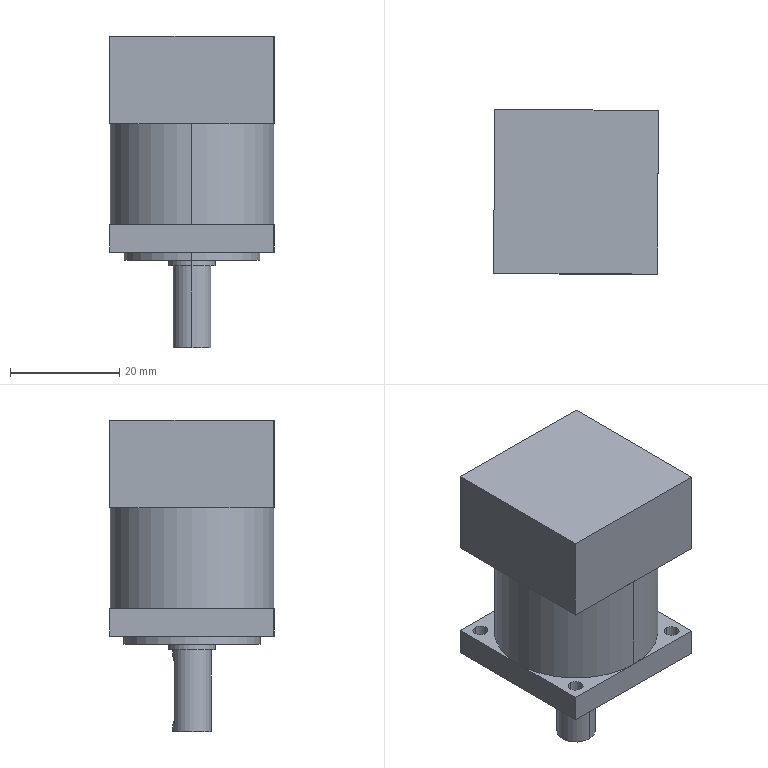Part | STEP file | 2026.6.15-Main Assembly图.sldasm-Part-97 | 1 solid | 44 faces | box 30.153 x 30.153 x 57 mm | volume 33186 mm3 | plane 24 | cylinder 20 | commonest cylinder face diameters 2.75 x8 2.5 x4 7 x2 8.5 x2 25 x2 30 x2
STEP:
#1=CARTESIAN_POINT('',(-1571.355,1394.756,3721.32));
#2=VERTEX_POINT('',#1);
#3=CARTESIAN_POINT('',(-1570.147,1394.755,3720.071));
#4=VERTEX_POINT('',#3);
#5=CARTESIAN_POINT('',(-1571.397,1394.756,3720.071));
#6=DIRECTION('',(0.0007664,1.,0.));
#7=DIRECTION('',(0.03353,-0.0000257,0.9994));
#8=AXIS2_PLACEMENT_3D('',#5,#6,#7);
#9=CIRCLE('',#8,1.25);
#10=EDGE_CURVE('',#2,#4,#9,.T.);
#11=ORIENTED_EDGE('',*,*,#10,.F.);
#12=CARTESIAN_POINT('',(-1571.354,1396.256,3721.32));
#13=VERTEX_POINT('',#12);
#14=CARTESIAN_POINT('',(-1571.354,1397.256,3721.32));
#15=DIRECTION('',(0.0007664,1.,0.));
#16=VECTOR('',#15,1000.);
#17=LINE('',#14,#16);
#18=EDGE_CURVE('',#2,#13,#17,.T.);
#19=ORIENTED_EDGE('',*,*,#18,.T.);
#20=CARTESIAN_POINT('',(-1570.146,1396.019,3720.071));
#21=VERTEX_POINT('',#20);
#22=CARTESIAN_POINT('',(-1570.146,1396.019,3720.071));
#23=CARTESIAN_POINT('',(-1570.146,1396.019,3720.234));
#24=CARTESIAN_POINT('',(-1570.178,1396.032,3720.394));
#25=CARTESIAN_POINT('',(-1570.299,1396.075,3720.691));
#26=CARTESIAN_POINT('',(-1570.388,1396.104,3720.826));
#27=CARTESIAN_POINT('',(-1570.608,1396.164,3721.054));
#28=CARTESIAN_POINT('',(-1570.741,1396.194,3721.147));
#29=CARTESIAN_POINT('',(-1571.031,1396.238,3721.277));
#30=CARTESIAN_POINT('',(-1571.192,1396.253,3721.315));
#31=CARTESIAN_POINT('',(-1571.354,1396.256,3721.32));
#32=B_SPLINE_CURVE_WITH_KNOTS('',3,(#22,#23,#24,#25,#26,#27,#28,#29,#30,#31),.UNSPECIFIED.,.F.,.F.,(4,2,2,2,4),(0.,0.0004821,0.0009642,0.001446,0.001928),.UNSPECIFIED.);
#33=EDGE_CURVE('',#21,#13,#32,.T.);
#34=ORIENTED_EDGE('',*,*,#33,.F.);
#35=CARTESIAN_POINT('',(-1570.145,1397.255,3720.071));
#36=DIRECTION('',(0.0007664,1.,0.));
#37=VECTOR('',#36,1000.);
#38=LINE('',#35,#37);
#39=EDGE_CURVE('',#4,#21,#38,.T.);
#40=ORIENTED_EDGE('',*,*,#39,.F.);
#41=EDGE_LOOP('',(#11,#19,#34,#40));
#42=FACE_OUTER_BOUND('',#41,.T.);
#43=CARTESIAN_POINT('',(-1571.395,1397.256,3720.071));
#44=DIRECTION('',(0.0007664,1.,0.));
#45=DIRECTION('',(0.03353,-0.0000257,0.9994));
#46=AXIS2_PLACEMENT_3D('',#43,#44,#45);
#47=CYLINDRICAL_SURFACE('',#46,1.25);
#48=ADVANCED_FACE('',(#42),#47,.F.);
#49=CARTESIAN_POINT('',(-1571.438,1396.256,3708.821));
#50=VERTEX_POINT('',#49);
#51=CARTESIAN_POINT('',(-1571.411,1396.256,3708.821));
#52=VERTEX_POINT('',#51);
#53=CARTESIAN_POINT('',(-1571.438,1396.256,3708.821));
#54=CARTESIAN_POINT('',(-1571.429,1396.256,3708.821));
#55=CARTESIAN_POINT('',(-1571.42,1396.256,3708.821));
#56=CARTESIAN_POINT('',(-1571.411,1396.256,3708.821));
#57=B_SPLINE_CURVE_WITH_KNOTS('',3,(#53,#54,#55,#56),.UNSPECIFIED.,.F.,.F.,(4,4),(-0.00004139,-0.00001499),.UNSPECIFIED.);
#58=EDGE_CURVE('',#50,#52,#57,.T.);
#59=ORIENTED_EDGE('',*,*,#58,.F.);
#60=CARTESIAN_POINT('',(-1571.439,1394.756,3708.821));
#61=VERTEX_POINT('',#60);
#62=CARTESIAN_POINT('',(-1571.437,1397.256,3708.821));
#63=DIRECTION('',(-0.0007664,-1.,0.));
#64=VECTOR('',#63,1000.);
#65=LINE('',#62,#64);
#66=EDGE_CURVE('',#50,#61,#65,.T.);
#67=ORIENTED_EDGE('',*,*,#66,.T.);
#68=CARTESIAN_POINT('',(-1570.147,1394.755,3710.071));
#69=VERTEX_POINT('',#68);
#70=CARTESIAN_POINT('',(-1571.397,1394.756,3710.071));
#71=DIRECTION('',(0.0007664,1.,0.));
#72=DIRECTION('',(0.03353,-0.0000257,0.9994));
#73=AXIS2_PLACEMENT_3D('',#70,#71,#72);
#74=CIRCLE('',#73,1.25);
#75=EDGE_CURVE('',#69,#61,#74,.T.);
#76=ORIENTED_EDGE('',*,*,#75,.F.);
#77=CARTESIAN_POINT('',(-1570.146,1396.019,3710.071));
#78=VERTEX_POINT('',#77);
#79=CARTESIAN_POINT('',(-1570.145,1397.255,3710.071));
#80=DIRECTION('',(-0.0007664,-1.,0.));
#81=VECTOR('',#80,1000.);
#82=LINE('',#79,#81);
#83=EDGE_CURVE('',#78,#69,#82,.T.);
#84=ORIENTED_EDGE('',*,*,#83,.F.);
#85=CARTESIAN_POINT('',(-1571.411,1396.256,3708.821));
#86=CARTESIAN_POINT('',(-1571.244,1396.256,3708.819));
#87=CARTESIAN_POINT('',(-1571.079,1396.244,3708.851));
#88=CARTESIAN_POINT('',(-1570.773,1396.201,3708.975));
#89=CARTESIAN_POINT('',(-1570.633,1396.17,3709.067));
#90=CARTESIAN_POINT('',(-1570.402,1396.109,3709.296));
#91=CARTESIAN_POINT('',(-1570.308,1396.078,3709.435));
#92=CARTESIAN_POINT('',(-1570.181,1396.033,3709.737));
#93=CARTESIAN_POINT('',(-1570.146,1396.019,3709.903));
#94=CARTESIAN_POINT('',(-1570.146,1396.019,3710.071));
#95=B_SPLINE_CURVE_WITH_KNOTS('',3,(#85,#86,#87,#88,#89,#90,#91,#92,#93,#94),.UNSPECIFIED.,.F.,.F.,(4,2,2,2,4),(-0.00001499,0.0004812,0.0009775,0.001474,0.00197),.UNSPECIFIED.);
#96=EDGE_CURVE('',#52,#78,#95,.T.);
#97=ORIENTED_EDGE('',*,*,#96,.F.);
#98=EDGE_LOOP('',(#59,#67,#76,#84,#97));
#99=FACE_OUTER_BOUND('',#98,.T.);
#100=CARTESIAN_POINT('',(-1571.395,1397.256,3710.071));
#101=DIRECTION('',(-0.0007664,-1.,0.));
#102=DIRECTION('',(-0.03353,0.0000257,-0.9994));
#103=AXIS2_PLACEMENT_3D('',#100,#101,#102);
#104=CYLINDRICAL_SURFACE('',#103,1.25);
#105=ADVANCED_FACE('',(#99),#104,.F.);
#106=CARTESIAN_POINT('',(-1571.405,1405.256,3725.071));
#107=VERTEX_POINT('',#106);
#108=CARTESIAN_POINT('',(-1571.424,1380.256,3725.071));
#109=VERTEX_POINT('',#108);
#110=CARTESIAN_POINT('',(-1571.414,1392.756,3725.071));
#111=DIRECTION('',(0.,0.,-1.));
#112=DIRECTION('',(1.,-0.005111,0.));
#113=AXIS2_PLACEMENT_3D('',#110,#111,#112);
#114=CIRCLE('',#113,12.5);
#115=EDGE_CURVE('',#107,#109,#114,.T.);
#116=ORIENTED_EDGE('',*,*,#115,.T.);
#117=CARTESIAN_POINT('',(-1571.424,1380.256,3723.571));
#118=VERTEX_POINT('',#117);
#119=CARTESIAN_POINT('',(-1571.424,1380.256,3725.071));
#120=DIRECTION('',(0.,0.,-1.));
#121=VECTOR('',#120,1000.);
#122=LINE('',#119,#121);
#123=EDGE_CURVE('',#109,#118,#122,.T.);
#124=ORIENTED_EDGE('',*,*,#123,.T.);
#125=CARTESIAN_POINT('',(-1571.405,1405.256,3723.571));
#126=VERTEX_POINT('',#125);
#127=CARTESIAN_POINT('',(-1571.414,1392.756,3723.571));
#128=DIRECTION('',(0.,0.,-1.));
#129=DIRECTION('',(1.,-0.005111,0.));
#130=AXIS2_PLACEMENT_3D('',#127,#128,#129);
#131=CIRCLE('',#130,12.5);
#132=EDGE_CURVE('',#126,#118,#131,.T.);
#133=ORIENTED_EDGE('',*,*,#132,.F.);
#134=CARTESIAN_POINT('',(-1571.405,1405.256,3725.071));
#135=DIRECTION('',(0.,0.,-1.));
#136=VECTOR('',#135,1000.);
#137=LINE('',#134,#136);
#138=EDGE_CURVE('',#107,#126,#137,.T.);
#139=ORIENTED_EDGE('',*,*,#138,.F.);
#140=EDGE_LOOP('',(#116,#124,#133,#139));
#141=FACE_OUTER_BOUND('',#140,.T.);
#142=CARTESIAN_POINT('',(-1571.414,1392.756,3725.071));
#143=DIRECTION('',(0.,0.,-1.));
#144=DIRECTION('',(0.0007664,1.,0.));
#145=AXIS2_PLACEMENT_3D('',#142,#143,#144);
#146=CYLINDRICAL_SURFACE('',#145,12.5);
#147=ADVANCED_FACE('',(#141),#146,.T.);
#148=CARTESIAN_POINT('',(-1571.426,1377.756,3748.571));
#149=VERTEX_POINT('',#148);
#150=CARTESIAN_POINT('',(-1556.414,1392.68,3748.571));
#151=VERTEX_POINT('',#150);
#152=CARTESIAN_POINT('',(-1571.414,1392.756,3748.571));
#153=DIRECTION('',(0.,0.,1.));
#154=DIRECTION('',(-0.0007664,-1.,0.));
#155=AXIS2_PLACEMENT_3D('',#152,#153,#154);
#156=CIRCLE('',#155,15.);
#157=EDGE_CURVE('',#149,#151,#156,.T.);
#158=ORIENTED_EDGE('',*,*,#157,.F.);
#159=CARTESIAN_POINT('',(-1571.426,1377.756,3730.071));
#160=VERTEX_POINT('',#159);
#161=CARTESIAN_POINT('',(-1571.426,1377.756,3748.571));
#162=DIRECTION('',(0.,0.,-1.));
#163=VECTOR('',#162,1000.);
#164=LINE('',#161,#163);
#165=EDGE_CURVE('',#149,#160,#164,.T.);
#166=ORIENTED_EDGE('',*,*,#165,.T.);
#167=CARTESIAN_POINT('',(-1556.414,1392.68,3730.071));
#168=VERTEX_POINT('',#167);
#169=CARTESIAN_POINT('',(-1571.414,1392.756,3730.071));
#170=DIRECTION('',(0.,0.,1.));
#171=DIRECTION('',(-0.0007664,-1.,0.));
#172=AXIS2_PLACEMENT_3D('',#169,#170,#171);
#173=CIRCLE('',#172,15.);
#174=EDGE_CURVE('',#160,#168,#173,.T.);
#175=ORIENTED_EDGE('',*,*,#174,.T.);
#176=CARTESIAN_POINT('',(-1571.337,1407.756,3730.071));
#177=VERTEX_POINT('',#176);
#178=CARTESIAN_POINT('',(-1571.414,1392.756,3730.071));
#179=DIRECTION('',(0.,0.,1.));
#180=DIRECTION('',(-0.0007664,-1.,0.));
#181=AXIS2_PLACEMENT_3D('',#178,#179,#180);
#182=CIRCLE('',#181,15.);
#183=EDGE_CURVE('',#168,#177,#182,.T.);
#184=ORIENTED_EDGE('',*,*,#183,.T.);
#185=CARTESIAN_POINT('',(-1571.403,1407.756,3730.071));
#186=VERTEX_POINT('',#185);
#187=CARTESIAN_POINT('',(-1571.414,1392.756,3730.071));
#188=DIRECTION('',(0.,0.,1.));
#189=DIRECTION('',(-0.0007664,-1.,0.));
#190=AXIS2_PLACEMENT_3D('',#187,#188,#189);
#191=CIRCLE('',#190,15.);
#192=EDGE_CURVE('',#177,#186,#191,.T.);
#193=ORIENTED_EDGE('',*,*,#192,.T.);
#194=CARTESIAN_POINT('',(-1571.403,1407.756,3748.571));
#195=VERTEX_POINT('',#194);
#196=CARTESIAN_POINT('',(-1571.403,1407.756,3748.571));
#197=DIRECTION('',(0.,0.,-1.));
#198=VECTOR('',#197,1000.);
#199=LINE('',#196,#198);
#200=EDGE_CURVE('',#195,#186,#199,.T.);
#201=ORIENTED_EDGE('',*,*,#200,.F.);
#202=CARTESIAN_POINT('',(-1571.337,1407.756,3748.571));
#203=VERTEX_POINT('',#202);
#204=CARTESIAN_POINT('',(-1571.414,1392.756,3748.571));
#205=DIRECTION('',(0.,0.,1.));
#206=DIRECTION('',(-0.0007664,-1.,0.));
#207=AXIS2_PLACEMENT_3D('',#204,#205,#206);
#208=CIRCLE('',#207,15.);
#209=EDGE_CURVE('',#203,#195,#208,.T.);
#210=ORIENTED_EDGE('',*,*,#209,.F.);
#211=CARTESIAN_POINT('',(-1571.414,1392.756,3748.571));
#212=DIRECTION('',(0.,0.,1.));
#213=DIRECTION('',(-0.0007664,-1.,0.));
#214=AXIS2_PLACEMENT_3D('',#211,#212,#213);
#215=CIRCLE('',#214,15.);
#216=EDGE_CURVE('',#151,#203,#215,.T.);
#217=ORIENTED_EDGE('',*,*,#216,.F.);
#218=EDGE_LOOP('',(#158,#166,#175,#184,#193,#201,#210,#217));
#219=FACE_OUTER_BOUND('',#218,.T.);
#220=CARTESIAN_POINT('',(-1571.414,1392.756,3748.571));
#221=DIRECTION('',(0.,0.,-1.));
#222=DIRECTION('',(0.0007664,1.,0.));
#223=AXIS2_PLACEMENT_3D('',#220,#221,#222);
#224=CYLINDRICAL_SURFACE('',#223,15.);
#225=ADVANCED_FACE('',(#219),#224,.T.);
#226=CARTESIAN_POINT('',(-1559.104,1378.944,3730.071));
#227=VERTEX_POINT('',#226);
#228=CARTESIAN_POINT('',(-1559.102,1381.694,3730.071));
#229=VERTEX_POINT('',#228);
#230=CARTESIAN_POINT('',(-1559.103,1380.319,3730.071));
#231=DIRECTION('',(0.,0.,-1.));
#232=DIRECTION('',(-1.,0.005111,0.));
#233=AXIS2_PLACEMENT_3D('',#230,#231,#232);
#234=CIRCLE('',#233,1.375);
#235=EDGE_CURVE('',#227,#229,#234,.T.);
#236=ORIENTED_EDGE('',*,*,#235,.F.);
#237=CARTESIAN_POINT('',(-1559.104,1378.944,3725.071));
#238=VERTEX_POINT('',#237);
#239=CARTESIAN_POINT('',(-1559.104,1378.944,3730.071));
#240=DIRECTION('',(0.,0.,-1.));
#241=VECTOR('',#240,1000.);
#242=LINE('',#239,#241);
#243=EDGE_CURVE('',#227,#238,#242,.T.);
#244=ORIENTED_EDGE('',*,*,#243,.T.);
#245=CARTESIAN_POINT('',(-1559.102,1381.694,3725.071));
#246=VERTEX_POINT('',#245);
#247=CARTESIAN_POINT('',(-1559.103,1380.319,3725.071));
#248=DIRECTION('',(0.,0.,-1.));
#249=DIRECTION('',(-1.,0.005111,0.));
#250=AXIS2_PLACEMENT_3D('',#247,#248,#249);
#251=CIRCLE('',#250,1.375);
#252=EDGE_CURVE('',#238,#246,#251,.T.);
#253=ORIENTED_EDGE('',*,*,#252,.T.);
#254=CARTESIAN_POINT('',(-1559.102,1381.694,3730.071));
#255=DIRECTION('',(0.,0.,-1.));
#256=VECTOR('',#255,1000.);
#257=LINE('',#254,#256);
#258=EDGE_CURVE('',#229,#246,#257,.T.);
#259=ORIENTED_EDGE('',*,*,#258,.F.);
#260=EDGE_LOOP('',(#236,#244,#253,#259));
#261=FACE_OUTER_BOUND('',#260,.T.);
#262=CARTESIAN_POINT('',(-1559.103,1380.319,3730.071));
#263=DIRECTION('',(0.,0.,-1.));
#264=DIRECTION('',(0.0007664,1.,0.));
#265=AXIS2_PLACEMENT_3D('',#262,#263,#264);
#266=CYLINDRICAL_SURFACE('',#265,1.375);
#267=ADVANCED_FACE('',(#261),#266,.F.);
#268=CARTESIAN_POINT('',(-1583.853,1379.07,3730.071));
#269=VERTEX_POINT('',#268);
#270=CARTESIAN_POINT('',(-1583.851,1381.82,3730.071));
#271=VERTEX_POINT('',#270);
#272=CARTESIAN_POINT('',(-1583.852,1380.445,3730.071));
#273=DIRECTION('',(0.,0.,-1.));
#274=DIRECTION('',(-1.,0.005111,0.));
#275=AXIS2_PLACEMENT_3D('',#272,#273,#274);
#276=CIRCLE('',#275,1.375);
#277=EDGE_CURVE('',#269,#271,#276,.T.);
#278=ORIENTED_EDGE('',*,*,#277,.F.);
#279=CARTESIAN_POINT('',(-1583.853,1379.07,3725.071));
#280=VERTEX_POINT('',#279);
#281=CARTESIAN_POINT('',(-1583.853,1379.07,3730.071));
#282=DIRECTION('',(0.,0.,-1.));
#283=VECTOR('',#282,1000.);
#284=LINE('',#281,#283);
#285=EDGE_CURVE('',#269,#280,#284,.T.);
#286=ORIENTED_EDGE('',*,*,#285,.T.);
#287=CARTESIAN_POINT('',(-1583.851,1381.82,3725.071));
#288=VERTEX_POINT('',#287);
#289=CARTESIAN_POINT('',(-1583.852,1380.445,3725.071));
#290=DIRECTION('',(0.,0.,-1.));
#291=DIRECTION('',(-1.,0.005111,0.));
#292=AXIS2_PLACEMENT_3D('',#289,#290,#291);
#293=CIRCLE('',#292,1.375);
#294=EDGE_CURVE('',#280,#288,#293,.T.);
#295=ORIENTED_EDGE('',*,*,#294,.T.);
#296=CARTESIAN_POINT('',(-1583.851,1381.82,3730.071));
#297=DIRECTION('',(0.,0.,-1.));
#298=VECTOR('',#297,1000.);
#299=LINE('',#296,#298);
#300=EDGE_CURVE('',#271,#288,#299,.T.);
#301=ORIENTED_EDGE('',*,*,#300,.F.);
#302=EDGE_LOOP('',(#278,#286,#295,#301));
#303=FACE_OUTER_BOUND('',#302,.T.);
#304=CARTESIAN_POINT('',(-1583.852,1380.445,3730.071));
#305=DIRECTION('',(0.,0.,-1.));
#306=DIRECTION('',(0.0007664,1.,0.));
#307=AXIS2_PLACEMENT_3D('',#304,#305,#306);
#308=CYLINDRICAL_SURFACE('',#307,1.375);
#309=ADVANCED_FACE('',(#303),#308,.F.);
#310=CARTESIAN_POINT('',(-1583.726,1403.819,3730.071));
#311=VERTEX_POINT('',#310);
#312=CARTESIAN_POINT('',(-1583.724,1406.569,3730.071));
#313=VERTEX_POINT('',#312);
#314=CARTESIAN_POINT('',(-1583.725,1405.194,3730.071));
#315=DIRECTION('',(0.,0.,-1.));
#316=DIRECTION('',(-1.,0.005111,0.));
#317=AXIS2_PLACEMENT_3D('',#314,#315,#316);
#318=CIRCLE('',#317,1.375);
#319=EDGE_CURVE('',#311,#313,#318,.T.);
#320=ORIENTED_EDGE('',*,*,#319,.F.);
#321=CARTESIAN_POINT('',(-1583.726,1403.819,3725.071));
#322=VERTEX_POINT('',#321);
#323=CARTESIAN_POINT('',(-1583.726,1403.819,3730.071));
#324=DIRECTION('',(0.,0.,-1.));
#325=VECTOR('',#324,1000.);
#326=LINE('',#323,#325);
#327=EDGE_CURVE('',#311,#322,#326,.T.);
#328=ORIENTED_EDGE('',*,*,#327,.T.);
#329=CARTESIAN_POINT('',(-1583.724,1406.569,3725.071));
#330=VERTEX_POINT('',#329);
#331=CARTESIAN_POINT('',(-1583.725,1405.194,3725.071));
#332=DIRECTION('',(0.,0.,-1.));
#333=DIRECTION('',(-1.,0.005111,0.));
#334=AXIS2_PLACEMENT_3D('',#331,#332,#333);
#335=CIRCLE('',#334,1.375);
#336=EDGE_CURVE('',#322,#330,#335,.T.);
#337=ORIENTED_EDGE('',*,*,#336,.T.);
#338=CARTESIAN_POINT('',(-1583.724,1406.569,3730.071));
#339=DIRECTION('',(0.,0.,-1.));
#340=VECTOR('',#339,1000.);
#341=LINE('',#338,#340);
#342=EDGE_CURVE('',#313,#330,#341,.T.);
#343=ORIENTED_EDGE('',*,*,#342,.F.);
#344=EDGE_LOOP('',(#320,#328,#337,#343));
#345=FACE_OUTER_BOUND('',#344,.T.);
#346=CARTESIAN_POINT('',(-1583.725,1405.194,3730.071));
#347=DIRECTION('',(0.,0.,-1.));
#348=DIRECTION('',(0.0007664,1.,0.));
#349=AXIS2_PLACEMENT_3D('',#346,#347,#348);
#350=CYLINDRICAL_SURFACE('',#349,1.375);
#351=ADVANCED_FACE('',(#345),#350,.F.);
#352=CARTESIAN_POINT('',(-1558.978,1403.692,3730.071));
#353=VERTEX_POINT('',#352);
#354=CARTESIAN_POINT('',(-1558.976,1406.442,3730.071));
#355=VERTEX_POINT('',#354);
#356=CARTESIAN_POINT('',(-1558.977,1405.067,3730.071));
#357=DIRECTION('',(0.,0.,-1.));
#358=DIRECTION('',(-1.,0.005111,0.));
#359=AXIS2_PLACEMENT_3D('',#356,#357,#358);
#360=CIRCLE('',#359,1.375);
#361=EDGE_CURVE('',#353,#355,#360,.T.);
#362=ORIENTED_EDGE('',*,*,#361,.F.);
#363=CARTESIAN_POINT('',(-1558.978,1403.692,3725.071));
#364=VERTEX_POINT('',#363);
#365=CARTESIAN_POINT('',(-1558.978,1403.692,3730.071));
#366=DIRECTION('',(0.,0.,-1.));
#367=VECTOR('',#366,1000.);
#368=LINE('',#365,#367);
#369=EDGE_CURVE('',#353,#364,#368,.T.);
#370=ORIENTED_EDGE('',*,*,#369,.T.);
#371=CARTESIAN_POINT('',(-1558.976,1406.442,3725.071));
#372=VERTEX_POINT('',#371);
#373=CARTESIAN_POINT('',(-1558.977,1405.067,3725.071));
#374=DIRECTION('',(0.,0.,-1.));
#375=DIRECTION('',(-1.,0.005111,0.));
#376=AXIS2_PLACEMENT_3D('',#373,#374,#375);
#377=CIRCLE('',#376,1.375);
#378=EDGE_CURVE('',#364,#372,#377,.T.);
#379=ORIENTED_EDGE('',*,*,#378,.T.);
#380=CARTESIAN_POINT('',(-1558.976,1406.442,3730.071));
#381=DIRECTION('',(0.,0.,-1.));
#382=VECTOR('',#381,1000.);
#383=LINE('',#380,#382);
#384=EDGE_CURVE('',#355,#372,#383,.T.);
#385=ORIENTED_EDGE('',*,*,#384,.F.);
#386=EDGE_LOOP('',(#362,#370,#379,#385));
#387=FACE_OUTER_BOUND('',#386,.T.);
#388=CARTESIAN_POINT('',(-1558.977,1405.067,3730.071));
#389=DIRECTION('',(0.,0.,-1.));
#390=DIRECTION('',(0.0007664,1.,0.));
#391=AXIS2_PLACEMENT_3D('',#388,#389,#390);
#392=CYLINDRICAL_SURFACE('',#391,1.375);
#393=ADVANCED_FACE('',(#387),#392,.F.);
#394=CARTESIAN_POINT('',(-1571.411,1397.006,3723.571));
#395=VERTEX_POINT('',#394);
#396=CARTESIAN_POINT('',(-1571.417,1388.506,3723.571));
#397=VERTEX_POINT('',#396);
#398=CARTESIAN_POINT('',(-1571.414,1392.756,3723.571));
#399=DIRECTION('',(0.,0.,-1.));
#400=DIRECTION('',(-1.,0.005111,0.));
#401=AXIS2_PLACEMENT_3D('',#398,#399,#400);
#402=CIRCLE('',#401,4.25);
#403=EDGE_CURVE('',#395,#397,#402,.T.);
#404=ORIENTED_EDGE('',*,*,#403,.T.);
#405=CARTESIAN_POINT('',(-1571.417,1388.506,3722.571));
#406=VERTEX_POINT('',#405);
#407=CARTESIAN_POINT('',(-1571.417,1388.506,3723.571));
#408=DIRECTION('',(0.,0.,-1.));
#409=VECTOR('',#408,1000.);
#410=LINE('',#407,#409);
#411=EDGE_CURVE('',#397,#406,#410,.T.);
#412=ORIENTED_EDGE('',*,*,#411,.T.);
#413=CARTESIAN_POINT('',(-1571.411,1397.006,3722.571));
#414=VERTEX_POINT('',#413);
#415=CARTESIAN_POINT('',(-1571.414,1392.756,3722.571));
#416=DIRECTION('',(0.,0.,-1.));
#417=DIRECTION('',(-1.,0.005111,0.));
#418=AXIS2_PLACEMENT_3D('',#415,#416,#417);
#419=CIRCLE('',#418,4.25);
#420=EDGE_CURVE('',#414,#406,#419,.T.);
#421=ORIENTED_EDGE('',*,*,#420,.F.);
#422=CARTESIAN_POINT('',(-1571.411,1397.006,3723.571));
#423=DIRECTION('',(0.,0.,-1.));
#424=VECTOR('',#423,1000.);
#425=LINE('',#422,#424);
#426=EDGE_CURVE('',#395,#414,#425,.T.);
#427=ORIENTED_EDGE('',*,*,#426,.F.);
#428=EDGE_LOOP('',(#404,#412,#421,#427));
#429=FACE_OUTER_BOUND('',#428,.T.);
#430=CARTESIAN_POINT('',(-1571.414,1392.756,3723.571));
#431=DIRECTION('',(0.,0.,-1.));
#432=DIRECTION('',(0.0007664,1.,0.));
#433=AXIS2_PLACEMENT_3D('',#430,#431,#432);
#434=CYLINDRICAL_SURFACE('',#433,4.25);
#435=ADVANCED_FACE('',(#429),#434,.T.);
#436=CARTESIAN_POINT('',(-1571.411,1396.256,3722.571));
#437=VERTEX_POINT('',#436);
#438=CARTESIAN_POINT('',(-1571.417,1389.256,3722.571));
#439=VERTEX_POINT('',#438);
#440=CARTESIAN_POINT('',(-1571.414,1392.756,3722.571));
#441=DIRECTION('',(0.,0.,-1.));
#442=DIRECTION('',(-1.,0.005111,0.));
#443=AXIS2_PLACEMENT_3D('',#440,#441,#442);
#444=CIRCLE('',#443,3.5);
#445=EDGE_CURVE('',#437,#439,#444,.T.);
#446=ORIENTED_EDGE('',*,*,#445,.T.);
#447=CARTESIAN_POINT('',(-1571.417,1389.256,3707.571));
#448=VERTEX_POINT('',#447);
#449=CARTESIAN_POINT('',(-1571.417,1389.256,3722.571));
#450=DIRECTION('',(0.,0.,-1.));
#451=VECTOR('',#450,1000.);
#452=LINE('',#449,#451);
#453=EDGE_CURVE('',#439,#448,#452,.T.);
#454=ORIENTED_EDGE('',*,*,#453,.T.);
#455=CARTESIAN_POINT('',(-1571.411,1396.256,3707.571));
#456=VERTEX_POINT('',#455);
#457=CARTESIAN_POINT('',(-1571.414,1392.756,3707.571));
#458=DIRECTION('',(0.,0.,-1.));
#459=DIRECTION('',(-1.,0.005111,0.));
#460=AXIS2_PLACEMENT_3D('',#457,#458,#459);
#461=CIRCLE('',#460,3.5);
#462=EDGE_CURVE('',#456,#448,#461,.T.);
#463=ORIENTED_EDGE('',*,*,#462,.F.);
#464=CARTESIAN_POINT('',(-1571.411,1396.256,3722.571));
#465=DIRECTION('',(0.,0.,-1.));
#466=VECTOR('',#465,1000.);
#467=LINE('',#464,#466);
#468=EDGE_CURVE('',#52,#456,#467,.T.);
#469=ORIENTED_EDGE('',*,*,#468,.F.);
#470=ORIENTED_EDGE('',*,*,#96,.T.);
#471=CARTESIAN_POINT('',(-1570.146,1396.019,3722.571));
#472=DIRECTION('',(0.,0.,1.));
#473=VECTOR('',#472,1000.);
#474=LINE('',#471,#473);
#475=EDGE_CURVE('',#78,#21,#474,.T.);
#476=ORIENTED_EDGE('',*,*,#475,.T.);
#477=ORIENTED_EDGE('',*,*,#33,.T.);
#478=CARTESIAN_POINT('',(-1571.411,1396.256,3721.321));
#479=VERTEX_POINT('',#478);
#480=CARTESIAN_POINT('',(-1571.354,1396.256,3721.32));
#481=CARTESIAN_POINT('',(-1571.373,1396.256,3721.321));
#482=CARTESIAN_POINT('',(-1571.392,1396.256,3721.321));
#483=CARTESIAN_POINT('',(-1571.411,1396.256,3721.321));
#484=B_SPLINE_CURVE_WITH_KNOTS('',3,(#480,#481,#482,#483),.UNSPECIFIED.,.F.,.F.,(4,4),(0.001928,0.001985),.UNSPECIFIED.);
#485=EDGE_CURVE('',#13,#479,#484,.T.);
#486=ORIENTED_EDGE('',*,*,#485,.T.);
#487=CARTESIAN_POINT('',(-1571.411,1396.256,3722.571));
#488=DIRECTION('',(0.,0.,-1.));
#489=VECTOR('',#488,1000.);
#490=LINE('',#487,#489);
#491=EDGE_CURVE('',#437,#479,#490,.T.);
#492=ORIENTED_EDGE('',*,*,#491,.F.);
#493=EDGE_LOOP('',(#446,#454,#463,#469,#470,#476,#477,#486,#492));
#494=FACE_OUTER_BOUND('',#493,.T.);
#495=CARTESIAN_POINT('',(-1571.414,1392.756,3722.571));
#496=DIRECTION('',(0.,0.,-1.));
#497=DIRECTION('',(0.0007664,1.,0.));
#498=AXIS2_PLACEMENT_3D('',#495,#496,#497);
#499=CYLINDRICAL_SURFACE('',#498,3.5);
#500=ADVANCED_FACE('',(#494),#499,.T.);
#501=ORIENTED_EDGE('',*,*,#453,.F.);
#502=CARTESIAN_POINT('',(-1571.414,1392.756,3722.571));
#503=DIRECTION('',(0.,0.,-1.));
#504=DIRECTION('',(-1.,0.005111,0.));
#505=AXIS2_PLACEMENT_3D('',#502,#503,#504);
#506=CIRCLE('',#505,3.5);
#507=EDGE_CURVE('',#439,#437,#506,.T.);
#508=ORIENTED_EDGE('',*,*,#507,.T.);
#509=ORIENTED_EDGE('',*,*,#491,.T.);
#510=CARTESIAN_POINT('',(-1572.646,1396.032,3720.071));
#511=VERTEX_POINT('',#510);
#512=CARTESIAN_POINT('',(-1571.411,1396.256,3721.321));
#513=CARTESIAN_POINT('',(-1571.576,1396.256,3721.319));
#514=CARTESIAN_POINT('',(-1571.738,1396.245,3721.284));
#515=CARTESIAN_POINT('',(-1572.037,1396.204,3721.156));
#516=CARTESIAN_POINT('',(-1572.173,1396.175,3721.063));
#517=CARTESIAN_POINT('',(-1572.398,1396.117,3720.835));
#518=CARTESIAN_POINT('',(-1572.49,1396.088,3720.698));
#519=CARTESIAN_POINT('',(-1572.613,1396.045,3720.4));
#520=CARTESIAN_POINT('',(-1572.646,1396.032,3720.236));
#521=CARTESIAN_POINT('',(-1572.646,1396.032,3720.071));
#522=B_SPLINE_CURVE_WITH_KNOTS('',3,(#512,#513,#514,#515,#516,#517,#518,#519,#520,#521),.UNSPECIFIED.,.F.,.F.,(4,2,2,2,4),(0.001985,0.002473,0.002962,0.00345,0.003938),.UNSPECIFIED.);
#523=EDGE_CURVE('',#479,#511,#522,.T.);
#524=ORIENTED_EDGE('',*,*,#523,.T.);
#525=CARTESIAN_POINT('',(-1572.646,1396.032,3710.071));
#526=VERTEX_POINT('',#525);
#527=CARTESIAN_POINT('',(-1572.646,1396.032,3722.571));
#528=DIRECTION('',(0.,0.,1.));
#529=VECTOR('',#528,1000.);
#530=LINE('',#527,#529);
#531=EDGE_CURVE('',#526,#511,#530,.T.);
#532=ORIENTED_EDGE('',*,*,#531,.F.);
#533=CARTESIAN_POINT('',(-1572.646,1396.032,3710.071));
#534=CARTESIAN_POINT('',(-1572.646,1396.032,3709.908));
#535=CARTESIAN_POINT('',(-1572.615,1396.045,3709.748));
#536=CARTESIAN_POINT('',(-1572.494,1396.086,3709.451));
#537=CARTESIAN_POINT('',(-1572.405,1396.115,3709.316));
#538=CARTESIAN_POINT('',(-1572.185,1396.172,3709.088));
#539=CARTESIAN_POINT('',(-1572.051,1396.201,3708.994));
#540=CARTESIAN_POINT('',(-1571.761,1396.242,3708.865));
#541=CARTESIAN_POINT('',(-1571.6,1396.255,3708.827));
#542=CARTESIAN_POINT('',(-1571.438,1396.256,3708.821));
#543=B_SPLINE_CURVE_WITH_KNOTS('',3,(#533,#534,#535,#536,#537,#538,#539,#540,#541,#542),.UNSPECIFIED.,.F.,.F.,(4,2,2,2,4),(-0.001969,-0.001487,-0.001005,-0.0005232,-0.00004139),.UNSPECIFIED.);
#544=EDGE_CURVE('',#526,#50,#543,.T.);
#545=ORIENTED_EDGE('',*,*,#544,.T.);
#546=ORIENTED_EDGE('',*,*,#58,.T.);
#547=ORIENTED_EDGE('',*,*,#468,.T.);
#548=CARTESIAN_POINT('',(-1571.414,1392.756,3707.571));
#549=DIRECTION('',(0.,0.,-1.));
#550=DIRECTION('',(-1.,0.005111,0.));
#551=AXIS2_PLACEMENT_3D('',#548,#549,#550);
#552=CIRCLE('',#551,3.5);
#553=EDGE_CURVE('',#448,#456,#552,.T.);
#554=ORIENTED_EDGE('',*,*,#553,.F.);
#555=EDGE_LOOP('',(#501,#508,#509,#524,#532,#545,#546,#547,#554));
#556=FACE_OUTER_BOUND('',#555,.T.);
#557=CARTESIAN_POINT('',(-1571.414,1392.756,3722.571));
#558=DIRECTION('',(0.,0.,-1.));
#559=DIRECTION('',(0.0007664,1.,0.));
#560=AXIS2_PLACEMENT_3D('',#557,#558,#559);
#561=CYLINDRICAL_SURFACE('',#560,3.5);
#562=ADVANCED_FACE('',(#556),#561,.T.);
#563=ORIENTED_EDGE('',*,*,#462,.T.);
#564=ORIENTED_EDGE('',*,*,#553,.T.);
#565=EDGE_LOOP('',(#563,#564));
#566=FACE_OUTER_BOUND('',#565,.T.);
#567=CARTESIAN_POINT('',(-1571.414,1392.756,3707.571));
#568=DIRECTION('',(0.,0.,-1.));
#569=DIRECTION('',(0.0007664,1.,0.));
#570=AXIS2_PLACEMENT_3D('',#567,#568,#569);
#571=PLANE('',#570);
#572=ADVANCED_FACE('',(#566),#571,.T.);
#573=ORIENTED_EDGE('',*,*,#411,.F.);
#574=CARTESIAN_POINT('',(-1571.414,1392.756,3723.571));
#575=DIRECTION('',(0.,0.,-1.));
#576=DIRECTION('',(-1.,0.005111,0.));
#577=AXIS2_PLACEMENT_3D('',#574,#575,#576);
#578=CIRCLE('',#577,4.25);
#579=EDGE_CURVE('',#397,#395,#578,.T.);
#580=ORIENTED_EDGE('',*,*,#579,.T.);
#581=ORIENTED_EDGE('',*,*,#426,.T.);
#582=CARTESIAN_POINT('',(-1571.414,1392.756,3722.571));
#583=DIRECTION('',(0.,0.,-1.));
#584=DIRECTION('',(-1.,0.005111,0.));
#585=AXIS2_PLACEMENT_3D('',#582,#583,#584);
#586=CIRCLE('',#585,4.25);
#587=EDGE_CURVE('',#406,#414,#586,.T.);
#588=ORIENTED_EDGE('',*,*,#587,.F.);
#589=EDGE_LOOP('',(#573,#580,#581,#588));
#590=FACE_OUTER_BOUND('',#589,.T.);
#591=CARTESIAN_POINT('',(-1571.414,1392.756,3723.571));
#592=DIRECTION('',(0.,0.,-1.));
#593=DIRECTION('',(0.0007664,1.,0.));
#594=AXIS2_PLACEMENT_3D('',#591,#592,#593);
#595=CYLINDRICAL_SURFACE('',#594,4.25);
#596=ADVANCED_FACE('',(#590),#595,.T.);
#597=ORIENTED_EDGE('',*,*,#445,.F.);
#598=ORIENTED_EDGE('',*,*,#507,.F.);
#599=EDGE_LOOP('',(#597,#598));
#600=FACE_BOUND('',#599,.T.);
#601=ORIENTED_EDGE('',*,*,#420,.T.);
#602=ORIENTED_EDGE('',*,*,#587,.T.);
#603=EDGE_LOOP('',(#601,#602));
#604=FACE_OUTER_BOUND('',#603,.T.);
#605=CARTESIAN_POINT('',(-1571.414,1392.756,3722.571));
#606=DIRECTION('',(0.,0.,1.));
#607=DIRECTION('',(-0.0007664,-1.,0.));
#608=AXIS2_PLACEMENT_3D('',#605,#606,#607);
#609=PLANE('',#608);
#610=ADVANCED_FACE('',(#600,#604),#609,.F.);
#611=ORIENTED_EDGE('',*,*,#183,.F.);
#612=CARTESIAN_POINT('',(-1556.338,1407.679,3730.071));
#613=VERTEX_POINT('',#612);
#614=CARTESIAN_POINT('',(-1556.338,1407.679,3730.071));
#615=DIRECTION('',(-0.005111,-1.,0.));
#616=VECTOR('',#615,1000.);
#617=LINE('',#614,#616);
#618=EDGE_CURVE('',#613,#168,#617,.T.);
#619=ORIENTED_EDGE('',*,*,#618,.F.);
#620=CARTESIAN_POINT('',(-1586.337,1407.833,3730.071));
#621=DIRECTION('',(1.,-0.005111,0.));
#622=VECTOR('',#621,1000.);
#623=LINE('',#620,#622);
#624=EDGE_CURVE('',#177,#613,#623,.T.);
#625=ORIENTED_EDGE('',*,*,#624,.F.);
#626=EDGE_LOOP('',(#611,#619,#625));
#627=FACE_OUTER_BOUND('',#626,.T.);
#628=CARTESIAN_POINT('',(-1558.977,1405.067,3730.071));
#629=DIRECTION('',(0.,0.,-1.));
#630=DIRECTION('',(-1.,0.005111,0.));
#631=AXIS2_PLACEMENT_3D('',#628,#629,#630);
#632=CIRCLE('',#631,1.375);
#633=EDGE_CURVE('',#355,#353,#632,.T.);
#634=ORIENTED_EDGE('',*,*,#633,.T.);
#635=ORIENTED_EDGE('',*,*,#361,.T.);
#636=EDGE_LOOP('',(#634,#635));
#637=FACE_BOUND('',#636,.T.);
#638=CARTESIAN_POINT('',(-1583.852,1380.445,3730.071));
#639=DIRECTION('',(0.,0.,-1.));
#640=DIRECTION('',(0.0007664,1.,0.));
#641=AXIS2_PLACEMENT_3D('',#638,#639,#640);
#642=PLANE('',#641);
#643=ADVANCED_FACE('',(#627,#637),#642,.F.);
#644=ORIENTED_EDGE('',*,*,#192,.F.);
#645=CARTESIAN_POINT('',(-1586.337,1407.833,3730.071));
#646=VERTEX_POINT('',#645);
#647=CARTESIAN_POINT('',(-1586.337,1407.833,3730.071));
#648=DIRECTION('',(1.,-0.005111,0.));
#649=VECTOR('',#648,1000.);
#650=LINE('',#647,#649);
#651=EDGE_CURVE('',#646,#177,#650,.T.);
#652=ORIENTED_EDGE('',*,*,#651,.F.);
#653=CARTESIAN_POINT('',(-1586.414,1392.833,3730.071));
#654=VERTEX_POINT('',#653);
#655=CARTESIAN_POINT('',(-1586.491,1377.833,3730.071));
#656=DIRECTION('',(0.005111,1.,0.));
#657=VECTOR('',#656,1000.);
#658=LINE('',#655,#657);
#659=EDGE_CURVE('',#654,#646,#658,.T.);
#660=ORIENTED_EDGE('',*,*,#659,.F.);
#661=CARTESIAN_POINT('',(-1571.414,1392.756,3730.071));
#662=DIRECTION('',(0.,0.,1.));
#663=DIRECTION('',(-0.0007664,-1.,0.));
#664=AXIS2_PLACEMENT_3D('',#661,#662,#663);
#665=CIRCLE('',#664,15.);
#666=EDGE_CURVE('',#186,#654,#665,.T.);
#667=ORIENTED_EDGE('',*,*,#666,.F.);
#668=EDGE_LOOP('',(#644,#652,#660,#667));
#669=FACE_OUTER_BOUND('',#668,.T.);
#670=CARTESIAN_POINT('',(-1583.725,1405.194,3730.071));
#671=DIRECTION('',(0.,0.,-1.));
#672=DIRECTION('',(-1.,0.005111,0.));
#673=AXIS2_PLACEMENT_3D('',#670,#671,#672);
#674=CIRCLE('',#673,1.375);
#675=EDGE_CURVE('',#313,#311,#674,.T.);
#676=ORIENTED_EDGE('',*,*,#675,.T.);
#677=ORIENTED_EDGE('',*,*,#319,.T.);
#678=EDGE_LOOP('',(#676,#677));
#679=FACE_BOUND('',#678,.T.);
#680=CARTESIAN_POINT('',(-1583.852,1380.445,3730.071));
#681=DIRECTION('',(0.,0.,-1.));
#682=DIRECTION('',(0.0007664,1.,0.));
#683=AXIS2_PLACEMENT_3D('',#680,#681,#682);
#684=PLANE('',#683);
#685=ADVANCED_FACE('',(#669,#679),#684,.F.);
#686=CARTESIAN_POINT('',(-1571.491,1377.757,3730.071));
#687=VERTEX_POINT('',#686);
#688=CARTESIAN_POINT('',(-1571.414,1392.756,3730.071));
#689=DIRECTION('',(0.,0.,1.));
#690=DIRECTION('',(-0.0007664,-1.,0.));
#691=AXIS2_PLACEMENT_3D('',#688,#689,#690);
#692=CIRCLE('',#691,15.);
#693=EDGE_CURVE('',#654,#687,#692,.T.);
#694=ORIENTED_EDGE('',*,*,#693,.F.);
#695=CARTESIAN_POINT('',(-1586.491,1377.833,3730.071));
#696=VERTEX_POINT('',#695);
#697=CARTESIAN_POINT('',(-1586.491,1377.833,3730.071));
#698=DIRECTION('',(0.005111,1.,0.));
#699=VECTOR('',#698,1000.);
#700=LINE('',#697,#699);
#701=EDGE_CURVE('',#696,#654,#700,.T.);
#702=ORIENTED_EDGE('',*,*,#701,.F.);
#703=CARTESIAN_POINT('',(-1556.491,1377.68,3730.071));
#704=DIRECTION('',(-1.,0.005111,0.));
#705=VECTOR('',#704,1000.);
#706=LINE('',#703,#705);
#707=EDGE_CURVE('',#687,#696,#706,.T.);
#708=ORIENTED_EDGE('',*,*,#707,.F.);
#709=EDGE_LOOP('',(#694,#702,#708));
#710=FACE_OUTER_BOUND('',#709,.T.);
#711=CARTESIAN_POINT('',(-1583.852,1380.445,3730.071));
#712=DIRECTION('',(0.,0.,-1.));
#713=DIRECTION('',(-1.,0.005111,0.));
#714=AXIS2_PLACEMENT_3D('',#711,#712,#713);
#715=CIRCLE('',#714,1.375);
#716=EDGE_CURVE('',#271,#269,#715,.T.);
#717=ORIENTED_EDGE('',*,*,#716,.T.);
#718=ORIENTED_EDGE('',*,*,#277,.T.);
#719=EDGE_LOOP('',(#717,#718));
#720=FACE_BOUND('',#719,.T.);
#721=CARTESIAN_POINT('',(-1583.852,1380.445,3730.071));
#722=DIRECTION('',(0.,0.,-1.));
#723=DIRECTION('',(0.0007664,1.,0.));
#724=AXIS2_PLACEMENT_3D('',#721,#722,#723);
#725=PLANE('',#724);
#726=ADVANCED_FACE('',(#710,#720),#725,.F.);
#727=CARTESIAN_POINT('',(-1586.337,1407.833,3725.071));
#728=VERTEX_POINT('',#727);
#729=CARTESIAN_POINT('',(-1556.338,1407.679,3725.071));
#730=VERTEX_POINT('',#729);
#731=CARTESIAN_POINT('',(-1586.337,1407.833,3725.071));
#732=DIRECTION('',(1.,-0.005111,0.));
#733=VECTOR('',#732,1000.);
#734=LINE('',#731,#733);
#735=EDGE_CURVE('',#728,#730,#734,.T.);
#736=ORIENTED_EDGE('',*,*,#735,.F.);
#737=CARTESIAN_POINT('',(-1586.337,1407.833,3730.071));
#738=DIRECTION('',(0.,0.,-1.));
#739=VECTOR('',#738,1000.);
#740=LINE('',#737,#739);
#741=EDGE_CURVE('',#646,#728,#740,.T.);
#742=ORIENTED_EDGE('',*,*,#741,.F.);
#743=ORIENTED_EDGE('',*,*,#651,.T.);
#744=ORIENTED_EDGE('',*,*,#624,.T.);
#745=CARTESIAN_POINT('',(-1556.338,1407.679,3730.071));
#746=DIRECTION('',(0.,0.,-1.));
#747=VECTOR('',#746,1000.);
#748=LINE('',#745,#747);
#749=EDGE_CURVE('',#613,#730,#748,.T.);
#750=ORIENTED_EDGE('',*,*,#749,.T.);
#751=EDGE_LOOP('',(#736,#742,#743,#744,#750));
#752=FACE_OUTER_BOUND('',#751,.T.);
#753=CARTESIAN_POINT('',(-1586.337,1407.833,3730.071));
#754=DIRECTION('',(0.005111,1.,0.));
#755=DIRECTION('',(0.03353,-0.0001714,0.9994));
#756=AXIS2_PLACEMENT_3D('',#753,#754,#755);
#757=PLANE('',#756);
#758=ADVANCED_FACE('',(#752),#757,.T.);
#759=CARTESIAN_POINT('',(-1556.491,1377.68,3725.071));
#760=VERTEX_POINT('',#759);
#761=CARTESIAN_POINT('',(-1556.338,1407.679,3725.071));
#762=DIRECTION('',(-0.005111,-1.,0.));
#763=VECTOR('',#762,1000.);
#764=LINE('',#761,#763);
#765=EDGE_CURVE('',#730,#760,#764,.T.);
#766=ORIENTED_EDGE('',*,*,#765,.F.);
#767=ORIENTED_EDGE('',*,*,#749,.F.);
#768=ORIENTED_EDGE('',*,*,#618,.T.);
#769=CARTESIAN_POINT('',(-1556.491,1377.68,3730.071));
#770=VERTEX_POINT('',#769);
#771=CARTESIAN_POINT('',(-1556.338,1407.679,3730.071));
#772=DIRECTION('',(-0.005111,-1.,0.));
#773=VECTOR('',#772,1000.);
#774=LINE('',#771,#773);
#775=EDGE_CURVE('',#168,#770,#774,.T.);
#776=ORIENTED_EDGE('',*,*,#775,.T.);
#777=CARTESIAN_POINT('',(-1556.491,1377.68,3730.071));
#778=DIRECTION('',(0.,0.,-1.));
#779=VECTOR('',#778,1000.);
#780=LINE('',#777,#779);
#781=EDGE_CURVE('',#770,#760,#780,.T.);
#782=ORIENTED_EDGE('',*,*,#781,.T.);
#783=EDGE_LOOP('',(#766,#767,#768,#776,#782));
#784=FACE_OUTER_BOUND('',#783,.T.);
#785=CARTESIAN_POINT('',(-1556.338,1407.679,3730.071));
#786=DIRECTION('',(1.,-0.005111,0.));
#787=DIRECTION('',(0.0006563,0.1284,-0.9917));
#788=AXIS2_PLACEMENT_3D('',#785,#786,#787);
#789=PLANE('',#788);
#790=ADVANCED_FACE('',(#784),#789,.T.);
#791=CARTESIAN_POINT('',(-1586.491,1377.833,3725.071));
#792=VERTEX_POINT('',#791);
#793=CARTESIAN_POINT('',(-1556.491,1377.68,3725.071));
#794=DIRECTION('',(-1.,0.005111,0.));
#795=VECTOR('',#794,1000.);
#796=LINE('',#793,#795);
#797=EDGE_CURVE('',#760,#792,#796,.T.);
#798=ORIENTED_EDGE('',*,*,#797,.F.);
#799=ORIENTED_EDGE('',*,*,#781,.F.);
#800=CARTESIAN_POINT('',(-1556.491,1377.68,3730.071));
#801=DIRECTION('',(-1.,0.005111,0.));
#802=VECTOR('',#801,1000.);
#803=LINE('',#800,#802);
#804=EDGE_CURVE('',#770,#687,#803,.T.);
#805=ORIENTED_EDGE('',*,*,#804,.T.);
#806=ORIENTED_EDGE('',*,*,#707,.T.);
#807=CARTESIAN_POINT('',(-1586.491,1377.833,3730.071));
#808=DIRECTION('',(0.,0.,-1.));
#809=VECTOR('',#808,1000.);
#810=LINE('',#807,#809);
#811=EDGE_CURVE('',#696,#792,#810,.T.);
#812=ORIENTED_EDGE('',*,*,#811,.T.);
#813=EDGE_LOOP('',(#798,#799,#805,#806,#812));
#814=FACE_OUTER_BOUND('',#813,.T.);
#815=CARTESIAN_POINT('',(-1556.491,1377.68,3730.071));
#816=DIRECTION('',(-0.005111,-1.,0.));
#817=DIRECTION('',(-0.03353,0.0001714,-0.9994));
#818=AXIS2_PLACEMENT_3D('',#815,#816,#817);
#819=PLANE('',#818);
#820=ADVANCED_FACE('',(#814),#819,.T.);
#821=ORIENTED_EDGE('',*,*,#369,.F.);
#822=ORIENTED_EDGE('',*,*,#633,.F.);
#823=ORIENTED_EDGE('',*,*,#384,.T.);
#824=CARTESIAN_POINT('',(-1558.977,1405.067,3725.071));
#825=DIRECTION('',(0.,0.,-1.));
#826=DIRECTION('',(-1.,0.005111,0.));
#827=AXIS2_PLACEMENT_3D('',#824,#825,#826);
#828=CIRCLE('',#827,1.375);
#829=EDGE_CURVE('',#372,#364,#828,.T.);
#830=ORIENTED_EDGE('',*,*,#829,.T.);
#831=EDGE_LOOP('',(#821,#822,#823,#830));
#832=FACE_OUTER_BOUND('',#831,.T.);
#833=CARTESIAN_POINT('',(-1558.977,1405.067,3730.071));
#834=DIRECTION('',(0.,0.,-1.));
#835=DIRECTION('',(0.0007664,1.,0.));
#836=AXIS2_PLACEMENT_3D('',#833,#834,#835);
#837=CYLINDRICAL_SURFACE('',#836,1.375);
#838=ADVANCED_FACE('',(#832),#837,.F.);
#839=ORIENTED_EDGE('',*,*,#327,.F.);
#840=ORIENTED_EDGE('',*,*,#675,.F.);
#841=ORIENTED_EDGE('',*,*,#342,.T.);
#842=CARTESIAN_POINT('',(-1583.725,1405.194,3725.071));
#843=DIRECTION('',(0.,0.,-1.));
#844=DIRECTION('',(-1.,0.005111,0.));
#845=AXIS2_PLACEMENT_3D('',#842,#843,#844);
#846=CIRCLE('',#845,1.375);
#847=EDGE_CURVE('',#330,#322,#846,.T.);
#848=ORIENTED_EDGE('',*,*,#847,.T.);
#849=EDGE_LOOP('',(#839,#840,#841,#848));
#850=FACE_OUTER_BOUND('',#849,.T.);
#851=CARTESIAN_POINT('',(-1583.725,1405.194,3730.071));
#852=DIRECTION('',(0.,0.,-1.));
#853=DIRECTION('',(0.0007664,1.,0.));
#854=AXIS2_PLACEMENT_3D('',#851,#852,#853);
#855=CYLINDRICAL_SURFACE('',#854,1.375);
#856=ADVANCED_FACE('',(#850),#855,.F.);
#857=ORIENTED_EDGE('',*,*,#285,.F.);
#858=ORIENTED_EDGE('',*,*,#716,.F.);
#859=ORIENTED_EDGE('',*,*,#300,.T.);
#860=CARTESIAN_POINT('',(-1583.852,1380.445,3725.071));
#861=DIRECTION('',(0.,0.,-1.));
#862=DIRECTION('',(-1.,0.005111,0.));
#863=AXIS2_PLACEMENT_3D('',#860,#861,#862);
#864=CIRCLE('',#863,1.375);
#865=EDGE_CURVE('',#288,#280,#864,.T.);
#866=ORIENTED_EDGE('',*,*,#865,.T.);
#867=EDGE_LOOP('',(#857,#858,#859,#866));
#868=FACE_OUTER_BOUND('',#867,.T.);
#869=CARTESIAN_POINT('',(-1583.852,1380.445,3730.071));
#870=DIRECTION('',(0.,0.,-1.));
#871=DIRECTION('',(0.0007664,1.,0.));
#872=AXIS2_PLACEMENT_3D('',#869,#870,#871);
#873=CYLINDRICAL_SURFACE('',#872,1.375);
#874=ADVANCED_FACE('',(#868),#873,.F.);
#875=CARTESIAN_POINT('',(-1586.491,1377.833,3725.071));
#876=DIRECTION('',(0.005111,1.,0.));
#877=VECTOR('',#876,1000.);
#878=LINE('',#875,#877);
#879=EDGE_CURVE('',#792,#728,#878,.T.);
#880=ORIENTED_EDGE('',*,*,#879,.F.);
#881=ORIENTED_EDGE('',*,*,#811,.F.);
#882=ORIENTED_EDGE('',*,*,#701,.T.);
#883=ORIENTED_EDGE('',*,*,#659,.T.);
#884=ORIENTED_EDGE('',*,*,#741,.T.);
#885=EDGE_LOOP('',(#880,#881,#882,#883,#884));
#886=FACE_OUTER_BOUND('',#885,.T.);
#887=CARTESIAN_POINT('',(-1586.491,1377.833,3730.071));
#888=DIRECTION('',(-1.,0.005111,0.));
#889=DIRECTION('',(-0.0006563,-0.1284,0.9917));
#890=AXIS2_PLACEMENT_3D('',#887,#888,#889);
#891=PLANE('',#890);
#892=ADVANCED_FACE('',(#886),#891,.T.);
#893=ORIENTED_EDGE('',*,*,#243,.F.);
#894=CARTESIAN_POINT('',(-1559.103,1380.319,3730.071));
#895=DIRECTION('',(0.,0.,-1.));
#896=DIRECTION('',(-1.,0.005111,0.));
#897=AXIS2_PLACEMENT_3D('',#894,#895,#896);
#898=CIRCLE('',#897,1.375);
#899=EDGE_CURVE('',#229,#227,#898,.T.);
#900=ORIENTED_EDGE('',*,*,#899,.F.);
#901=ORIENTED_EDGE('',*,*,#258,.T.);
#902=CARTESIAN_POINT('',(-1559.103,1380.319,3725.071));
#903=DIRECTION('',(0.,0.,-1.));
#904=DIRECTION('',(-1.,0.005111,0.));
#905=AXIS2_PLACEMENT_3D('',#902,#903,#904);
#906=CIRCLE('',#905,1.375);
#907=EDGE_CURVE('',#246,#238,#906,.T.);
#908=ORIENTED_EDGE('',*,*,#907,.T.);
#909=EDGE_LOOP('',(#893,#900,#901,#908));
#910=FACE_OUTER_BOUND('',#909,.T.);
#911=CARTESIAN_POINT('',(-1559.103,1380.319,3730.071));
#912=DIRECTION('',(0.,0.,-1.));
#913=DIRECTION('',(0.0007664,1.,0.));
#914=AXIS2_PLACEMENT_3D('',#911,#912,#913);
#915=CYLINDRICAL_SURFACE('',#914,1.375);
#916=ADVANCED_FACE('',(#910),#915,.F.);
#917=CARTESIAN_POINT('',(-1571.414,1392.756,3730.071));
#918=DIRECTION('',(0.,0.,1.));
#919=DIRECTION('',(-0.0007664,-1.,0.));
#920=AXIS2_PLACEMENT_3D('',#917,#918,#919);
#921=CIRCLE('',#920,15.);
#922=EDGE_CURVE('',#687,#160,#921,.T.);
#923=ORIENTED_EDGE('',*,*,#922,.F.);
#924=ORIENTED_EDGE('',*,*,#804,.F.);
#925=ORIENTED_EDGE('',*,*,#775,.F.);
#926=ORIENTED_EDGE('',*,*,#174,.F.);
#927=EDGE_LOOP('',(#923,#924,#925,#926));
#928=FACE_OUTER_BOUND('',#927,.T.);
#929=ORIENTED_EDGE('',*,*,#899,.T.);
#930=ORIENTED_EDGE('',*,*,#235,.T.);
#931=EDGE_LOOP('',(#929,#930));
#932=FACE_BOUND('',#931,.T.);
#933=CARTESIAN_POINT('',(-1583.852,1380.445,3730.071));
#934=DIRECTION('',(0.,0.,-1.));
#935=DIRECTION('',(0.0007664,1.,0.));
#936=AXIS2_PLACEMENT_3D('',#933,#934,#935);
#937=PLANE('',#936);
#938=ADVANCED_FACE('',(#928,#932),#937,.F.);
#939=ORIENTED_EDGE('',*,*,#115,.F.);
#940=CARTESIAN_POINT('',(-1571.414,1392.756,3725.071));
#941=DIRECTION('',(0.,0.,-1.));
#942=DIRECTION('',(1.,-0.005111,0.));
#943=AXIS2_PLACEMENT_3D('',#940,#941,#942);
#944=CIRCLE('',#943,12.5);
#945=EDGE_CURVE('',#109,#107,#944,.T.);
#946=ORIENTED_EDGE('',*,*,#945,.F.);
#947=EDGE_LOOP('',(#939,#946));
#948=FACE_BOUND('',#947,.T.);
#949=ORIENTED_EDGE('',*,*,#735,.T.);
#950=ORIENTED_EDGE('',*,*,#765,.T.);
#951=ORIENTED_EDGE('',*,*,#797,.T.);
#952=ORIENTED_EDGE('',*,*,#879,.T.);
#953=EDGE_LOOP('',(#949,#950,#951,#952));
#954=FACE_OUTER_BOUND('',#953,.T.);
#955=ORIENTED_EDGE('',*,*,#865,.F.);
#956=ORIENTED_EDGE('',*,*,#294,.F.);
#957=EDGE_LOOP('',(#955,#956));
#958=FACE_BOUND('',#957,.T.);
#959=ORIENTED_EDGE('',*,*,#847,.F.);
#960=ORIENTED_EDGE('',*,*,#336,.F.);
#961=EDGE_LOOP('',(#959,#960));
#962=FACE_BOUND('',#961,.T.);
#963=ORIENTED_EDGE('',*,*,#829,.F.);
#964=ORIENTED_EDGE('',*,*,#378,.F.);
#965=EDGE_LOOP('',(#963,#964));
#966=FACE_BOUND('',#965,.T.);
#967=ORIENTED_EDGE('',*,*,#907,.F.);
#968=ORIENTED_EDGE('',*,*,#252,.F.);
#969=EDGE_LOOP('',(#967,#968));
#970=FACE_BOUND('',#969,.T.);
#971=CARTESIAN_POINT('',(-1583.852,1380.445,3725.071));
#972=DIRECTION('',(0.,0.,-1.));
#973=DIRECTION('',(0.0007664,1.,0.));
#974=AXIS2_PLACEMENT_3D('',#971,#972,#973);
#975=PLANE('',#974);
#976=ADVANCED_FACE('',(#948,#954,#958,#962,#966,#970),#975,.T.);
#977=CARTESIAN_POINT('',(-1556.338,1407.679,3748.571));
#978=VERTEX_POINT('',#977);
#979=CARTESIAN_POINT('',(-1556.491,1377.68,3748.571));
#980=DIRECTION('',(0.005111,1.,0.));
#981=VECTOR('',#980,1000.);
#982=LINE('',#979,#981);
#983=EDGE_CURVE('',#151,#978,#982,.T.);
#984=ORIENTED_EDGE('',*,*,#983,.F.);
#985=ORIENTED_EDGE('',*,*,#216,.T.);
#986=CARTESIAN_POINT('',(-1556.338,1407.679,3748.571));
#987=DIRECTION('',(-1.,0.005111,0.));
#988=VECTOR('',#987,1000.);
#989=LINE('',#986,#988);
#990=EDGE_CURVE('',#978,#203,#989,.T.);
#991=ORIENTED_EDGE('',*,*,#990,.F.);
#992=EDGE_LOOP('',(#984,#985,#991));
#993=FACE_OUTER_BOUND('',#992,.T.);
#994=CARTESIAN_POINT('',(-1598.52,785.116,3748.571));
#995=DIRECTION('',(0.,0.,1.));
#996=DIRECTION('',(-0.0007664,-1.,0.));
#997=AXIS2_PLACEMENT_3D('',#994,#995,#996);
#998=PLANE('',#997);
#999=ADVANCED_FACE('',(#993),#998,.F.);
#1000=CARTESIAN_POINT('',(-1586.337,1407.833,3748.571));
#1001=VERTEX_POINT('',#1000);
#1002=CARTESIAN_POINT('',(-1556.338,1407.679,3748.571));
#1003=DIRECTION('',(-1.,0.005111,0.));
#1004=VECTOR('',#1003,1000.);
#1005=LINE('',#1002,#1004);
#1006=EDGE_CURVE('',#203,#1001,#1005,.T.);
#1007=ORIENTED_EDGE('',*,*,#1006,.F.);
#1008=ORIENTED_EDGE('',*,*,#209,.T.);
#1009=CARTESIAN_POINT('',(-1586.414,1392.833,3748.571));
#1010=VERTEX_POINT('',#1009);
#1011=CARTESIAN_POINT('',(-1571.414,1392.756,3748.571));
#1012=DIRECTION('',(0.,0.,1.));
#1013=DIRECTION('',(-0.0007664,-1.,0.));
#1014=AXIS2_PLACEMENT_3D('',#1011,#1012,#1013);
#1015=CIRCLE('',#1014,15.);
#1016=EDGE_CURVE('',#195,#1010,#1015,.T.);
#1017=ORIENTED_EDGE('',*,*,#1016,.T.);
#1018=CARTESIAN_POINT('',(-1586.337,1407.833,3748.571));
#1019=DIRECTION('',(-0.005111,-1.,0.));
#1020=VECTOR('',#1019,1000.);
#1021=LINE('',#1018,#1020);
#1022=EDGE_CURVE('',#1001,#1010,#1021,.T.);
#1023=ORIENTED_EDGE('',*,*,#1022,.F.);
#1024=EDGE_LOOP('',(#1007,#1008,#1017,#1023));
#1025=FACE_OUTER_BOUND('',#1024,.T.);
#1026=CARTESIAN_POINT('',(-1598.52,785.116,3748.571));
#1027=DIRECTION('',(0.,0.,1.));
#1028=DIRECTION('',(-0.0007664,-1.,0.));
#1029=AXIS2_PLACEMENT_3D('',#1026,#1027,#1028);
#1030=PLANE('',#1029);
#1031=ADVANCED_FACE('',(#1025),#1030,.F.);
#1032=CARTESIAN_POINT('',(-1586.491,1377.833,3748.571));
#1033=VERTEX_POINT('',#1032);
#1034=CARTESIAN_POINT('',(-1586.337,1407.833,3748.571));
#1035=DIRECTION('',(-0.005111,-1.,0.));
#1036=VECTOR('',#1035,1000.);
#1037=LINE('',#1034,#1036);
#1038=EDGE_CURVE('',#1010,#1033,#1037,.T.);
#1039=ORIENTED_EDGE('',*,*,#1038,.F.);
#1040=CARTESIAN_POINT('',(-1571.491,1377.757,3748.571));
#1041=VERTEX_POINT('',#1040);
#1042=CARTESIAN_POINT('',(-1571.414,1392.756,3748.571));
#1043=DIRECTION('',(0.,0.,1.));
#1044=DIRECTION('',(-0.0007664,-1.,0.));
#1045=AXIS2_PLACEMENT_3D('',#1042,#1043,#1044);
#1046=CIRCLE('',#1045,15.);
#1047=EDGE_CURVE('',#1010,#1041,#1046,.T.);
#1048=ORIENTED_EDGE('',*,*,#1047,.T.);
#1049=CARTESIAN_POINT('',(-1586.491,1377.833,3748.571));
#1050=DIRECTION('',(1.,-0.005111,0.));
#1051=VECTOR('',#1050,1000.);
#1052=LINE('',#1049,#1051);
#1053=EDGE_CURVE('',#1033,#1041,#1052,.T.);
#1054=ORIENTED_EDGE('',*,*,#1053,.F.);
#1055=EDGE_LOOP('',(#1039,#1048,#1054));
#1056=FACE_OUTER_BOUND('',#1055,.T.);
#1057=CARTESIAN_POINT('',(-1598.52,785.116,3748.571));
#1058=DIRECTION('',(0.,0.,1.));
#1059=DIRECTION('',(-0.0007664,-1.,0.));
#1060=AXIS2_PLACEMENT_3D('',#1057,#1058,#1059);
#1061=PLANE('',#1060);
#1062=ADVANCED_FACE('',(#1056),#1061,.F.);
#1063=ORIENTED_EDGE('',*,*,#990,.T.);
#1064=ORIENTED_EDGE('',*,*,#1006,.T.);
#1065=CARTESIAN_POINT('',(-1586.337,1407.833,3764.571));
#1066=VERTEX_POINT('',#1065);
#1067=CARTESIAN_POINT('',(-1586.337,1407.833,3764.571));
#1068=DIRECTION('',(0.,0.,-1.));
#1069=VECTOR('',#1068,1000.);
#1070=LINE('',#1067,#1069);
#1071=EDGE_CURVE('',#1066,#1001,#1070,.T.);
#1072=ORIENTED_EDGE('',*,*,#1071,.F.);
#1073=CARTESIAN_POINT('',(-1556.338,1407.679,3764.571));
#1074=VERTEX_POINT('',#1073);
#1075=CARTESIAN_POINT('',(-1556.338,1407.679,3764.571));
#1076=DIRECTION('',(-1.,0.005111,0.));
#1077=VECTOR('',#1076,1000.);
#1078=LINE('',#1075,#1077);
#1079=EDGE_CURVE('',#1074,#1066,#1078,.T.);
#1080=ORIENTED_EDGE('',*,*,#1079,.F.);
#1081=CARTESIAN_POINT('',(-1556.338,1407.679,3764.571));
#1082=DIRECTION('',(0.,0.,-1.));
#1083=VECTOR('',#1082,1000.);
#1084=LINE('',#1081,#1083);
#1085=EDGE_CURVE('',#1074,#978,#1084,.T.);
#1086=ORIENTED_EDGE('',*,*,#1085,.T.);
#1087=EDGE_LOOP('',(#1063,#1064,#1072,#1080,#1086));
#1088=FACE_OUTER_BOUND('',#1087,.T.);
#1089=CARTESIAN_POINT('',(-1556.338,1407.679,3764.571));
#1090=DIRECTION('',(-0.005111,-1.,0.));
#1091=DIRECTION('',(-0.03353,0.0001714,-0.9994));
#1092=AXIS2_PLACEMENT_3D('',#1089,#1090,#1091);
#1093=PLANE('',#1092);
#1094=ADVANCED_FACE('',(#1088),#1093,.F.);
#1095=ORIENTED_EDGE('',*,*,#1022,.T.);
#1096=ORIENTED_EDGE('',*,*,#1038,.T.);
#1097=CARTESIAN_POINT('',(-1586.491,1377.833,3764.571));
#1098=VERTEX_POINT('',#1097);
#1099=CARTESIAN_POINT('',(-1586.491,1377.833,3764.571));
#1100=DIRECTION('',(0.,0.,-1.));
#1101=VECTOR('',#1100,1000.);
#1102=LINE('',#1099,#1101);
#1103=EDGE_CURVE('',#1098,#1033,#1102,.T.);
#1104=ORIENTED_EDGE('',*,*,#1103,.F.);
#1105=CARTESIAN_POINT('',(-1586.337,1407.833,3764.571));
#1106=DIRECTION('',(-0.005111,-1.,0.));
#1107=VECTOR('',#1106,1000.);
#1108=LINE('',#1105,#1107);
#1109=EDGE_CURVE('',#1066,#1098,#1108,.T.);
#1110=ORIENTED_EDGE('',*,*,#1109,.F.);
#1111=ORIENTED_EDGE('',*,*,#1071,.T.);
#1112=EDGE_LOOP('',(#1095,#1096,#1104,#1110,#1111));
#1113=FACE_OUTER_BOUND('',#1112,.T.);
#1114=CARTESIAN_POINT('',(-1586.337,1407.833,3764.571));
#1115=DIRECTION('',(1.,-0.005111,0.));
#1116=DIRECTION('',(0.0006563,0.1284,-0.9917));
#1117=AXIS2_PLACEMENT_3D('',#1114,#1115,#1116);
#1118=PLANE('',#1117);
#1119=ADVANCED_FACE('',(#1113),#1118,.F.);
#1120=ORIENTED_EDGE('',*,*,#1053,.T.);
#1121=CARTESIAN_POINT('',(-1556.491,1377.68,3748.571));
#1122=VERTEX_POINT('',#1121);
#1123=CARTESIAN_POINT('',(-1586.491,1377.833,3748.571));
#1124=DIRECTION('',(1.,-0.005111,0.));
#1125=VECTOR('',#1124,1000.);
#1126=LINE('',#1123,#1125);
#1127=EDGE_CURVE('',#1041,#1122,#1126,.T.);
#1128=ORIENTED_EDGE('',*,*,#1127,.T.);
#1129=CARTESIAN_POINT('',(-1556.491,1377.68,3764.571));
#1130=VERTEX_POINT('',#1129);
#1131=CARTESIAN_POINT('',(-1556.491,1377.68,3764.571));
#1132=DIRECTION('',(0.,0.,-1.));
#1133=VECTOR('',#1132,1000.);
#1134=LINE('',#1131,#1133);
#1135=EDGE_CURVE('',#1130,#1122,#1134,.T.);
#1136=ORIENTED_EDGE('',*,*,#1135,.F.);
#1137=CARTESIAN_POINT('',(-1586.491,1377.833,3764.571));
#1138=DIRECTION('',(1.,-0.005111,0.));
#1139=VECTOR('',#1138,1000.);
#1140=LINE('',#1137,#1139);
#1141=EDGE_CURVE('',#1098,#1130,#1140,.T.);
#1142=ORIENTED_EDGE('',*,*,#1141,.F.);
#1143=ORIENTED_EDGE('',*,*,#1103,.T.);
#1144=EDGE_LOOP('',(#1120,#1128,#1136,#1142,#1143));
#1145=FACE_OUTER_BOUND('',#1144,.T.);
#1146=CARTESIAN_POINT('',(-1586.491,1377.833,3764.571));
#1147=DIRECTION('',(0.005111,1.,0.));
#1148=DIRECTION('',(0.03353,-0.0001714,0.9994));
#1149=AXIS2_PLACEMENT_3D('',#1146,#1147,#1148);
#1150=PLANE('',#1149);
#1151=ADVANCED_FACE('',(#1145),#1150,.F.);
#1152=CARTESIAN_POINT('',(-1556.491,1377.68,3748.571));
#1153=DIRECTION('',(0.005111,1.,0.));
#1154=VECTOR('',#1153,1000.);
#1155=LINE('',#1152,#1154);
#1156=EDGE_CURVE('',#1122,#151,#1155,.T.);
#1157=ORIENTED_EDGE('',*,*,#1156,.T.);
#1158=ORIENTED_EDGE('',*,*,#983,.T.);
#1159=ORIENTED_EDGE('',*,*,#1085,.F.);
#1160=CARTESIAN_POINT('',(-1556.491,1377.68,3764.571));
#1161=DIRECTION('',(0.005111,1.,0.));
#1162=VECTOR('',#1161,1000.);
#1163=LINE('',#1160,#1162);
#1164=EDGE_CURVE('',#1130,#1074,#1163,.T.);
#1165=ORIENTED_EDGE('',*,*,#1164,.F.);
#1166=ORIENTED_EDGE('',*,*,#1135,.T.);
#1167=EDGE_LOOP('',(#1157,#1158,#1159,#1165,#1166));
#1168=FACE_OUTER_BOUND('',#1167,.T.);
#1169=CARTESIAN_POINT('',(-1556.491,1377.68,3764.571));
#1170=DIRECTION('',(-1.,0.005111,0.));
#1171=DIRECTION('',(-0.0006563,-0.1284,0.9917));
#1172=AXIS2_PLACEMENT_3D('',#1169,#1170,#1171);
#1173=PLANE('',#1172);
#1174=ADVANCED_FACE('',(#1168),#1173,.F.);
#1175=ORIENTED_EDGE('',*,*,#1079,.T.);
#1176=ORIENTED_EDGE('',*,*,#1109,.T.);
#1177=ORIENTED_EDGE('',*,*,#1141,.T.);
#1178=ORIENTED_EDGE('',*,*,#1164,.T.);
#1179=EDGE_LOOP('',(#1175,#1176,#1177,#1178));
#1180=FACE_OUTER_BOUND('',#1179,.T.);
#1181=CARTESIAN_POINT('',(-1598.52,785.116,3764.571));
#1182=DIRECTION('',(0.,0.,1.));
#1183=DIRECTION('',(-0.0007664,-1.,0.));
#1184=AXIS2_PLACEMENT_3D('',#1181,#1182,#1183);
#1185=PLANE('',#1184);
#1186=ADVANCED_FACE('',(#1180),#1185,.T.);
#1187=ORIENTED_EDGE('',*,*,#1127,.F.);
#1188=CARTESIAN_POINT('',(-1571.414,1392.756,3748.571));
#1189=DIRECTION('',(0.,0.,1.));
#1190=DIRECTION('',(-0.0007664,-1.,0.));
#1191=AXIS2_PLACEMENT_3D('',#1188,#1189,#1190);
#1192=CIRCLE('',#1191,15.);
#1193=EDGE_CURVE('',#1041,#149,#1192,.T.);
#1194=ORIENTED_EDGE('',*,*,#1193,.T.);
#1195=ORIENTED_EDGE('',*,*,#157,.T.);
#1196=ORIENTED_EDGE('',*,*,#1156,.F.);
#1197=EDGE_LOOP('',(#1187,#1194,#1195,#1196));
#1198=FACE_OUTER_BOUND('',#1197,.T.);
#1199=CARTESIAN_POINT('',(-1598.52,785.116,3748.571));
#1200=DIRECTION('',(0.,0.,1.));
#1201=DIRECTION('',(-0.0007664,-1.,0.));
#1202=AXIS2_PLACEMENT_3D('',#1199,#1200,#1201);
#1203=PLANE('',#1202);
#1204=ADVANCED_FACE('',(#1198),#1203,.F.);
#1205=ORIENTED_EDGE('',*,*,#165,.F.);
#1206=ORIENTED_EDGE('',*,*,#1193,.F.);
#1207=ORIENTED_EDGE('',*,*,#1047,.F.);
#1208=ORIENTED_EDGE('',*,*,#1016,.F.);
#1209=ORIENTED_EDGE('',*,*,#200,.T.);
#1210=ORIENTED_EDGE('',*,*,#666,.T.);
#1211=ORIENTED_EDGE('',*,*,#693,.T.);
#1212=ORIENTED_EDGE('',*,*,#922,.T.);
#1213=EDGE_LOOP('',(#1205,#1206,#1207,#1208,#1209,#1210,#1211,#1212));
#1214=FACE_OUTER_BOUND('',#1213,.T.);
#1215=CARTESIAN_POINT('',(-1571.414,1392.756,3748.571));
#1216=DIRECTION('',(0.,0.,-1.));
#1217=DIRECTION('',(0.0007664,1.,0.));
#1218=AXIS2_PLACEMENT_3D('',#1215,#1216,#1217);
#1219=CYLINDRICAL_SURFACE('',#1218,15.);
#1220=ADVANCED_FACE('',(#1214),#1219,.T.);
#1221=ORIENTED_EDGE('',*,*,#123,.F.);
#1222=ORIENTED_EDGE('',*,*,#945,.T.);
#1223=ORIENTED_EDGE('',*,*,#138,.T.);
#1224=CARTESIAN_POINT('',(-1571.414,1392.756,3723.571));
#1225=DIRECTION('',(0.,0.,-1.));
#1226=DIRECTION('',(1.,-0.005111,0.));
#1227=AXIS2_PLACEMENT_3D('',#1224,#1225,#1226);
#1228=CIRCLE('',#1227,12.5);
#1229=EDGE_CURVE('',#118,#126,#1228,.T.);
#1230=ORIENTED_EDGE('',*,*,#1229,.F.);
#1231=EDGE_LOOP('',(#1221,#1222,#1223,#1230));
#1232=FACE_OUTER_BOUND('',#1231,.T.);
#1233=CARTESIAN_POINT('',(-1571.414,1392.756,3725.071));
#1234=DIRECTION('',(0.,0.,-1.));
#1235=DIRECTION('',(0.0007664,1.,0.));
#1236=AXIS2_PLACEMENT_3D('',#1233,#1234,#1235);
#1237=CYLINDRICAL_SURFACE('',#1236,12.5);
#1238=ADVANCED_FACE('',(#1232),#1237,.T.);
#1239=ORIENTED_EDGE('',*,*,#403,.F.);
#1240=ORIENTED_EDGE('',*,*,#579,.F.);
#1241=EDGE_LOOP('',(#1239,#1240));
#1242=FACE_BOUND('',#1241,.T.);
#1243=ORIENTED_EDGE('',*,*,#132,.T.);
#1244=ORIENTED_EDGE('',*,*,#1229,.T.);
#1245=EDGE_LOOP('',(#1243,#1244));
#1246=FACE_OUTER_BOUND('',#1245,.T.);
#1247=CARTESIAN_POINT('',(-1571.414,1392.756,3723.571));
#1248=DIRECTION('',(0.,0.,-1.));
#1249=DIRECTION('',(0.0007664,1.,0.));
#1250=AXIS2_PLACEMENT_3D('',#1247,#1248,#1249);
#1251=PLANE('',#1250);
#1252=ADVANCED_FACE('',(#1242,#1246),#1251,.T.);
#1253=CARTESIAN_POINT('',(-1570.147,1394.755,3721.321));
#1254=DIRECTION('',(0.,0.,1.));
#1255=VECTOR('',#1254,1000.);
#1256=LINE('',#1253,#1255);
#1257=EDGE_CURVE('',#69,#4,#1256,.T.);
#1258=ORIENTED_EDGE('',*,*,#1257,.F.);
#1259=ORIENTED_EDGE('',*,*,#75,.T.);
#1260=CARTESIAN_POINT('',(-1572.647,1394.757,3710.071));
#1261=VERTEX_POINT('',#1260);
#1262=CARTESIAN_POINT('',(-1571.397,1394.756,3710.071));
#1263=DIRECTION('',(0.0007664,1.,0.));
#1264=DIRECTION('',(0.03353,-0.0000257,0.9994));
#1265=AXIS2_PLACEMENT_3D('',#1262,#1263,#1264);
#1266=CIRCLE('',#1265,1.25);
#1267=EDGE_CURVE('',#61,#1261,#1266,.T.);
#1268=ORIENTED_EDGE('',*,*,#1267,.T.);
#1269=CARTESIAN_POINT('',(-1572.647,1394.757,3720.071));
#1270=VERTEX_POINT('',#1269);
#1271=CARTESIAN_POINT('',(-1572.647,1394.757,3721.321));
#1272=DIRECTION('',(0.,0.,1.));
#1273=VECTOR('',#1272,1000.);
#1274=LINE('',#1271,#1273);
#1275=EDGE_CURVE('',#1261,#1270,#1274,.T.);
#1276=ORIENTED_EDGE('',*,*,#1275,.T.);
#1277=CARTESIAN_POINT('',(-1571.397,1394.756,3720.071));
#1278=DIRECTION('',(0.0007664,1.,0.));
#1279=DIRECTION('',(0.03353,-0.0000257,0.9994));
#1280=AXIS2_PLACEMENT_3D('',#1277,#1278,#1279);
#1281=CIRCLE('',#1280,1.25);
#1282=EDGE_CURVE('',#1270,#2,#1281,.T.);
#1283=ORIENTED_EDGE('',*,*,#1282,.T.);
#1284=ORIENTED_EDGE('',*,*,#10,.T.);
#1285=EDGE_LOOP('',(#1258,#1259,#1268,#1276,#1283,#1284));
#1286=FACE_OUTER_BOUND('',#1285,.T.);
#1287=CARTESIAN_POINT('',(-1571.397,1394.756,3721.321));
#1288=DIRECTION('',(0.0007664,1.,0.));
#1289=DIRECTION('',(0.,0.,-1.));
#1290=AXIS2_PLACEMENT_3D('',#1287,#1288,#1289);
#1291=PLANE('',#1290);
#1292=ADVANCED_FACE('',(#1286),#1291,.T.);
#1293=ORIENTED_EDGE('',*,*,#1275,.F.);
#1294=CARTESIAN_POINT('',(-1572.646,1396.032,3710.071));
#1295=DIRECTION('',(0.0007664,1.,0.));
#1296=VECTOR('',#1295,1000.);
#1297=LINE('',#1294,#1296);
#1298=EDGE_CURVE('',#1261,#526,#1297,.T.);
#1299=ORIENTED_EDGE('',*,*,#1298,.T.);
#1300=ORIENTED_EDGE('',*,*,#531,.T.);
#1301=CARTESIAN_POINT('',(-1572.647,1394.757,3720.071));
#1302=DIRECTION('',(-0.0007664,-1.,0.));
#1303=VECTOR('',#1302,1000.);
#1304=LINE('',#1301,#1303);
#1305=EDGE_CURVE('',#511,#1270,#1304,.T.);
#1306=ORIENTED_EDGE('',*,*,#1305,.T.);
#1307=EDGE_LOOP('',(#1293,#1299,#1300,#1306));
#1308=FACE_OUTER_BOUND('',#1307,.T.);
#1309=CARTESIAN_POINT('',(-1572.645,1397.257,3721.321));
#1310=DIRECTION('',(-1.,0.0007664,0.));
#1311=DIRECTION('',(-0.00009842,-0.1284,0.9917));
#1312=AXIS2_PLACEMENT_3D('',#1309,#1310,#1311);
#1313=PLANE('',#1312);
#1314=ADVANCED_FACE('',(#1308),#1313,.F.);
#1315=ORIENTED_EDGE('',*,*,#475,.F.);
#1316=ORIENTED_EDGE('',*,*,#83,.T.);
#1317=ORIENTED_EDGE('',*,*,#1257,.T.);
#1318=ORIENTED_EDGE('',*,*,#39,.T.);
#1319=EDGE_LOOP('',(#1315,#1316,#1317,#1318));
#1320=FACE_OUTER_BOUND('',#1319,.T.);
#1321=CARTESIAN_POINT('',(-1570.145,1397.255,3721.321));
#1322=DIRECTION('',(-1.,0.0007664,0.));
#1323=DIRECTION('',(-0.00009842,-0.1284,0.9917));
#1324=AXIS2_PLACEMENT_3D('',#1321,#1322,#1323);
#1325=PLANE('',#1324);
#1326=ADVANCED_FACE('',(#1320),#1325,.T.);
#1327=ORIENTED_EDGE('',*,*,#66,.F.);
#1328=ORIENTED_EDGE('',*,*,#544,.F.);
#1329=ORIENTED_EDGE('',*,*,#1298,.F.);
#1330=ORIENTED_EDGE('',*,*,#1267,.F.);
#1331=EDGE_LOOP('',(#1327,#1328,#1329,#1330));
#1332=FACE_OUTER_BOUND('',#1331,.T.);
#1333=CARTESIAN_POINT('',(-1571.395,1397.256,3710.071));
#1334=DIRECTION('',(-0.0007664,-1.,0.));
#1335=DIRECTION('',(-0.03353,0.0000257,-0.9994));
#1336=AXIS2_PLACEMENT_3D('',#1333,#1334,#1335);
#1337=CYLINDRICAL_SURFACE('',#1336,1.25);
#1338=ADVANCED_FACE('',(#1332),#1337,.F.);
#1339=ORIENTED_EDGE('',*,*,#18,.F.);
#1340=ORIENTED_EDGE('',*,*,#1282,.F.);
#1341=ORIENTED_EDGE('',*,*,#1305,.F.);
#1342=ORIENTED_EDGE('',*,*,#523,.F.);
#1343=ORIENTED_EDGE('',*,*,#485,.F.);
#1344=EDGE_LOOP('',(#1339,#1340,#1341,#1342,#1343));
#1345=FACE_OUTER_BOUND('',#1344,.T.);
#1346=CARTESIAN_POINT('',(-1571.395,1397.256,3720.071));
#1347=DIRECTION('',(0.0007664,1.,0.));
#1348=DIRECTION('',(0.03353,-0.0000257,0.9994));
#1349=AXIS2_PLACEMENT_3D('',#1346,#1347,#1348);
#1350=CYLINDRICAL_SURFACE('',#1349,1.25);
#1351=ADVANCED_FACE('',(#1345),#1350,.F.);
#1352=CLOSED_SHELL('',(#48,#105,#147,#225,#267,#309,#351,#393,#435,#500,#562,#572,#596,#610,#643,#685,#726,#758,#790,#820,#838,#856,#874,#892,#916,#938,#976,#999,#1031,#1062,#1094,#1119,#1151,#1174,#1186,#1204,#1220,#1238,#1252,#1292,#1314,#1326,#1338,#1351));
#1353=MANIFOLD_SOLID_BREP('',#1352);
#1354=CARTESIAN_POINT('',(0.,0.,0.));
#1355=DIRECTION('',(0.,0.,1.));
#1356=DIRECTION('',(1.,0.,0.));
#1357=AXIS2_PLACEMENT_3D('',#1354,#1355,#1356);
#1358=(LENGTH_UNIT()NAMED_UNIT(*)SI_UNIT(.MILLI.,.METRE.));
#1359=UNCERTAINTY_MEASURE_WITH_UNIT(LENGTH_MEASURE(0.00001),#1358,'','');
#1360=(NAMED_UNIT(*)PLANE_ANGLE_UNIT()SI_UNIT($,.RADIAN.));
#1361=(NAMED_UNIT(*)SI_UNIT($,.STERADIAN.)SOLID_ANGLE_UNIT());
#1362=(GEOMETRIC_REPRESENTATION_CONTEXT(3)GLOBAL_UNCERTAINTY_ASSIGNED_CONTEXT((#1359))GLOBAL_UNIT_ASSIGNED_CONTEXT((#1358,#1360,#1361))REPRESENTATION_CONTEXT('',''));
#1363=ADVANCED_BREP_SHAPE_REPRESENTATION('',(#1353,#1357),#1362);